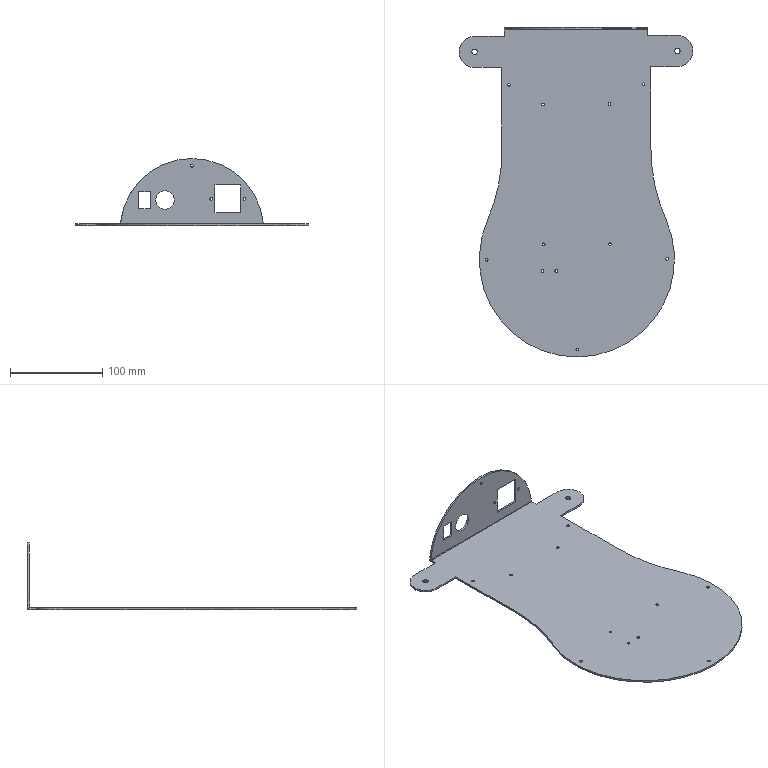Part | SolidWorks | features BaseBody 1 | 1 solid | 66 faces | box 253.998 x 358.292 x 72.88 mm | volume 141546 mm3 | cylinder 44 | plane 22 | commonest cylinder face diameters 3 x28 6 x4 34 x3 20 x2 211.992 x2 378.008 x2